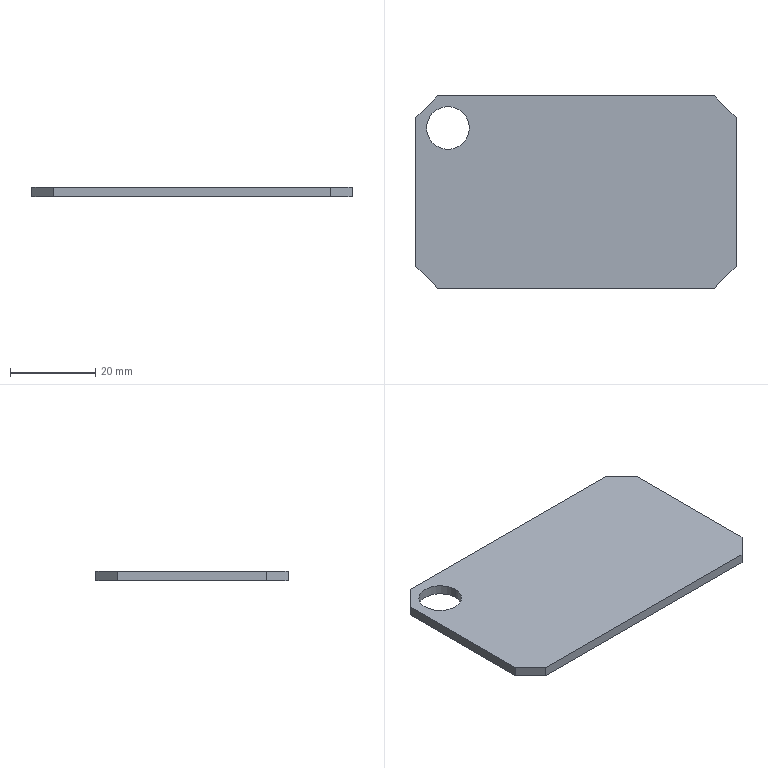Part | STEP file | [20]-1 | 1 solid | 12 faces | box 75 x 45 x 2.3 mm | volume 7467 mm3 | plane 10 | cylinder 2 | commonest cylinder face diameters 10 x2
STEP:
#1=CARTESIAN_POINT('',(2.5,37.5,0.));
#2=VERTEX_POINT('',#1);
#3=CARTESIAN_POINT('',(12.5,37.5,0.));
#4=VERTEX_POINT('',#3);
#5=CARTESIAN_POINT('',(7.5,37.5,0.));
#6=DIRECTION('',(0.,0.,1.));
#7=DIRECTION('',(1.,0.,0.));
#8=AXIS2_PLACEMENT_3D('',#5,#6,#7);
#9=CIRCLE('',#8,5.);
#10=EDGE_CURVE('',#2,#4,#9,.T.);
#11=ORIENTED_EDGE('',*,*,#10,.F.);
#12=CARTESIAN_POINT('',(2.5,37.5,2.3));
#13=VERTEX_POINT('',#12);
#14=CARTESIAN_POINT('',(2.5,37.5,0.));
#15=DIRECTION('',(0.,0.,1.));
#16=VECTOR('',#15,1000.);
#17=LINE('',#14,#16);
#18=EDGE_CURVE('',#2,#13,#17,.T.);
#19=ORIENTED_EDGE('',*,*,#18,.T.);
#20=CARTESIAN_POINT('',(12.5,37.5,2.3));
#21=VERTEX_POINT('',#20);
#22=CARTESIAN_POINT('',(7.5,37.5,2.3));
#23=DIRECTION('',(0.,0.,-1.));
#24=DIRECTION('',(-1.,0.,0.));
#25=AXIS2_PLACEMENT_3D('',#22,#23,#24);
#26=CIRCLE('',#25,5.);
#27=EDGE_CURVE('',#21,#13,#26,.T.);
#28=ORIENTED_EDGE('',*,*,#27,.F.);
#29=CARTESIAN_POINT('',(12.5,37.5,0.));
#30=DIRECTION('',(0.,0.,1.));
#31=VECTOR('',#30,1000.);
#32=LINE('',#29,#31);
#33=EDGE_CURVE('',#4,#21,#32,.T.);
#34=ORIENTED_EDGE('',*,*,#33,.F.);
#35=EDGE_LOOP('',(#11,#19,#28,#34));
#36=FACE_OUTER_BOUND('',#35,.T.);
#37=CARTESIAN_POINT('',(7.5,37.5,0.));
#38=DIRECTION('',(0.,0.,1.));
#39=DIRECTION('',(1.,0.,0.));
#40=AXIS2_PLACEMENT_3D('',#37,#38,#39);
#41=CYLINDRICAL_SURFACE('',#40,5.);
#42=ADVANCED_FACE('',(#36),#41,.F.);
#43=ORIENTED_EDGE('',*,*,#27,.T.);
#44=CARTESIAN_POINT('',(7.5,37.5,2.3));
#45=DIRECTION('',(0.,0.,-1.));
#46=DIRECTION('',(-1.,0.,0.));
#47=AXIS2_PLACEMENT_3D('',#44,#45,#46);
#48=CIRCLE('',#47,5.);
#49=EDGE_CURVE('',#13,#21,#48,.T.);
#50=ORIENTED_EDGE('',*,*,#49,.T.);
#51=EDGE_LOOP('',(#43,#50));
#52=FACE_BOUND('',#51,.T.);
#53=CARTESIAN_POINT('',(0.,5.,2.3));
#54=VERTEX_POINT('',#53);
#55=CARTESIAN_POINT('',(0.,40.,2.3));
#56=VERTEX_POINT('',#55);
#57=CARTESIAN_POINT('',(0.,22.5,2.3));
#58=DIRECTION('',(0.,1.,0.));
#59=VECTOR('',#58,1000.);
#60=LINE('',#57,#59);
#61=EDGE_CURVE('',#54,#56,#60,.T.);
#62=ORIENTED_EDGE('',*,*,#61,.F.);
#63=CARTESIAN_POINT('',(5.,0.,2.3));
#64=VERTEX_POINT('',#63);
#65=CARTESIAN_POINT('',(10.,-5.,2.3));
#66=DIRECTION('',(0.7071,-0.7071,0.));
#67=VECTOR('',#66,1000.);
#68=LINE('',#65,#67);
#69=EDGE_CURVE('',#54,#64,#68,.T.);
#70=ORIENTED_EDGE('',*,*,#69,.T.);
#71=CARTESIAN_POINT('',(70.,0.,2.3));
#72=VERTEX_POINT('',#71);
#73=CARTESIAN_POINT('',(37.5,0.,2.3));
#74=DIRECTION('',(-1.,0.,0.));
#75=VECTOR('',#74,1000.);
#76=LINE('',#73,#75);
#77=EDGE_CURVE('',#72,#64,#76,.T.);
#78=ORIENTED_EDGE('',*,*,#77,.F.);
#79=CARTESIAN_POINT('',(75.,5.,2.3));
#80=VERTEX_POINT('',#79);
#81=CARTESIAN_POINT('',(65.,-5.,2.3));
#82=DIRECTION('',(0.7071,0.7071,0.));
#83=VECTOR('',#82,1000.);
#84=LINE('',#81,#83);
#85=EDGE_CURVE('',#72,#80,#84,.T.);
#86=ORIENTED_EDGE('',*,*,#85,.T.);
#87=CARTESIAN_POINT('',(75.,40.,2.3));
#88=VERTEX_POINT('',#87);
#89=CARTESIAN_POINT('',(75.,22.5,2.3));
#90=DIRECTION('',(0.,-1.,0.));
#91=VECTOR('',#90,1000.);
#92=LINE('',#89,#91);
#93=EDGE_CURVE('',#88,#80,#92,.T.);
#94=ORIENTED_EDGE('',*,*,#93,.F.);
#95=CARTESIAN_POINT('',(70.,45.,2.3));
#96=VERTEX_POINT('',#95);
#97=CARTESIAN_POINT('',(65.,50.,2.3));
#98=DIRECTION('',(-0.7071,0.7071,0.));
#99=VECTOR('',#98,1000.);
#100=LINE('',#97,#99);
#101=EDGE_CURVE('',#88,#96,#100,.T.);
#102=ORIENTED_EDGE('',*,*,#101,.T.);
#103=CARTESIAN_POINT('',(5.,45.,2.3));
#104=VERTEX_POINT('',#103);
#105=CARTESIAN_POINT('',(37.5,45.,2.3));
#106=DIRECTION('',(1.,0.,0.));
#107=VECTOR('',#106,1000.);
#108=LINE('',#105,#107);
#109=EDGE_CURVE('',#104,#96,#108,.T.);
#110=ORIENTED_EDGE('',*,*,#109,.F.);
#111=CARTESIAN_POINT('',(10.,50.,2.3));
#112=DIRECTION('',(-0.7071,-0.7071,0.));
#113=VECTOR('',#112,1000.);
#114=LINE('',#111,#113);
#115=EDGE_CURVE('',#104,#56,#114,.T.);
#116=ORIENTED_EDGE('',*,*,#115,.T.);
#117=EDGE_LOOP('',(#62,#70,#78,#86,#94,#102,#110,#116));
#118=FACE_OUTER_BOUND('',#117,.T.);
#119=CARTESIAN_POINT('',(37.5,22.5,2.3));
#120=DIRECTION('',(0.,0.,1.));
#121=DIRECTION('',(0.,1.,0.));
#122=AXIS2_PLACEMENT_3D('',#119,#120,#121);
#123=PLANE('',#122);
#124=ADVANCED_FACE('',(#52,#118),#123,.T.);
#125=CARTESIAN_POINT('',(75.,5.,0.));
#126=VERTEX_POINT('',#125);
#127=CARTESIAN_POINT('',(75.,40.,0.));
#128=VERTEX_POINT('',#127);
#129=CARTESIAN_POINT('',(75.,22.5,0.));
#130=DIRECTION('',(0.,1.,0.));
#131=VECTOR('',#130,1000.);
#132=LINE('',#129,#131);
#133=EDGE_CURVE('',#126,#128,#132,.T.);
#134=ORIENTED_EDGE('',*,*,#133,.T.);
#135=CARTESIAN_POINT('',(75.,40.,0.));
#136=DIRECTION('',(0.,0.,1.));
#137=VECTOR('',#136,1000.);
#138=LINE('',#135,#137);
#139=EDGE_CURVE('',#128,#88,#138,.T.);
#140=ORIENTED_EDGE('',*,*,#139,.T.);
#141=ORIENTED_EDGE('',*,*,#93,.T.);
#142=CARTESIAN_POINT('',(75.,5.,0.));
#143=DIRECTION('',(0.,0.,-1.));
#144=VECTOR('',#143,1000.);
#145=LINE('',#142,#144);
#146=EDGE_CURVE('',#80,#126,#145,.T.);
#147=ORIENTED_EDGE('',*,*,#146,.T.);
#148=EDGE_LOOP('',(#134,#140,#141,#147));
#149=FACE_OUTER_BOUND('',#148,.T.);
#150=CARTESIAN_POINT('',(75.,22.5,0.));
#151=DIRECTION('',(1.,0.,0.));
#152=DIRECTION('',(0.,0.,-1.));
#153=AXIS2_PLACEMENT_3D('',#150,#151,#152);
#154=PLANE('',#153);
#155=ADVANCED_FACE('',(#149),#154,.T.);
#156=ORIENTED_EDGE('',*,*,#77,.T.);
#157=CARTESIAN_POINT('',(5.,0.,0.));
#158=VERTEX_POINT('',#157);
#159=CARTESIAN_POINT('',(5.,0.,0.));
#160=DIRECTION('',(0.,0.,-1.));
#161=VECTOR('',#160,1000.);
#162=LINE('',#159,#161);
#163=EDGE_CURVE('',#64,#158,#162,.T.);
#164=ORIENTED_EDGE('',*,*,#163,.T.);
#165=CARTESIAN_POINT('',(70.,0.,0.));
#166=VERTEX_POINT('',#165);
#167=CARTESIAN_POINT('',(37.5,0.,0.));
#168=DIRECTION('',(1.,0.,0.));
#169=VECTOR('',#168,1000.);
#170=LINE('',#167,#169);
#171=EDGE_CURVE('',#158,#166,#170,.T.);
#172=ORIENTED_EDGE('',*,*,#171,.T.);
#173=CARTESIAN_POINT('',(70.,0.,0.));
#174=DIRECTION('',(0.,0.,1.));
#175=VECTOR('',#174,1000.);
#176=LINE('',#173,#175);
#177=EDGE_CURVE('',#166,#72,#176,.T.);
#178=ORIENTED_EDGE('',*,*,#177,.T.);
#179=EDGE_LOOP('',(#156,#164,#172,#178));
#180=FACE_OUTER_BOUND('',#179,.T.);
#181=CARTESIAN_POINT('',(37.5,0.,0.));
#182=DIRECTION('',(0.,-1.,0.));
#183=DIRECTION('',(0.,0.,1.));
#184=AXIS2_PLACEMENT_3D('',#181,#182,#183);
#185=PLANE('',#184);
#186=ADVANCED_FACE('',(#180),#185,.T.);
#187=CARTESIAN_POINT('',(0.,40.,0.));
#188=VERTEX_POINT('',#187);
#189=CARTESIAN_POINT('',(0.,5.,0.));
#190=VERTEX_POINT('',#189);
#191=CARTESIAN_POINT('',(0.,22.5,0.));
#192=DIRECTION('',(0.,-1.,0.));
#193=VECTOR('',#192,1000.);
#194=LINE('',#191,#193);
#195=EDGE_CURVE('',#188,#190,#194,.T.);
#196=ORIENTED_EDGE('',*,*,#195,.T.);
#197=CARTESIAN_POINT('',(0.,5.,0.));
#198=DIRECTION('',(0.,0.,1.));
#199=VECTOR('',#198,1000.);
#200=LINE('',#197,#199);
#201=EDGE_CURVE('',#190,#54,#200,.T.);
#202=ORIENTED_EDGE('',*,*,#201,.T.);
#203=ORIENTED_EDGE('',*,*,#61,.T.);
#204=CARTESIAN_POINT('',(0.,40.,0.));
#205=DIRECTION('',(0.,0.,-1.));
#206=VECTOR('',#205,1000.);
#207=LINE('',#204,#206);
#208=EDGE_CURVE('',#56,#188,#207,.T.);
#209=ORIENTED_EDGE('',*,*,#208,.T.);
#210=EDGE_LOOP('',(#196,#202,#203,#209));
#211=FACE_OUTER_BOUND('',#210,.T.);
#212=CARTESIAN_POINT('',(0.,22.5,0.));
#213=DIRECTION('',(-1.,0.,0.));
#214=DIRECTION('',(0.,0.,1.));
#215=AXIS2_PLACEMENT_3D('',#212,#213,#214);
#216=PLANE('',#215);
#217=ADVANCED_FACE('',(#211),#216,.T.);
#218=CARTESIAN_POINT('',(7.5,37.5,0.));
#219=DIRECTION('',(0.,0.,1.));
#220=DIRECTION('',(1.,0.,0.));
#221=AXIS2_PLACEMENT_3D('',#218,#219,#220);
#222=CIRCLE('',#221,5.);
#223=EDGE_CURVE('',#4,#2,#222,.T.);
#224=ORIENTED_EDGE('',*,*,#223,.T.);
#225=ORIENTED_EDGE('',*,*,#10,.T.);
#226=EDGE_LOOP('',(#224,#225));
#227=FACE_BOUND('',#226,.T.);
#228=ORIENTED_EDGE('',*,*,#171,.F.);
#229=CARTESIAN_POINT('',(10.,-5.,0.));
#230=DIRECTION('',(-0.7071,0.7071,0.));
#231=VECTOR('',#230,1000.);
#232=LINE('',#229,#231);
#233=EDGE_CURVE('',#158,#190,#232,.T.);
#234=ORIENTED_EDGE('',*,*,#233,.T.);
#235=ORIENTED_EDGE('',*,*,#195,.F.);
#236=CARTESIAN_POINT('',(5.,45.,0.));
#237=VERTEX_POINT('',#236);
#238=CARTESIAN_POINT('',(10.,50.,0.));
#239=DIRECTION('',(0.7071,0.7071,0.));
#240=VECTOR('',#239,1000.);
#241=LINE('',#238,#240);
#242=EDGE_CURVE('',#188,#237,#241,.T.);
#243=ORIENTED_EDGE('',*,*,#242,.T.);
#244=CARTESIAN_POINT('',(70.,45.,0.));
#245=VERTEX_POINT('',#244);
#246=CARTESIAN_POINT('',(37.5,45.,0.));
#247=DIRECTION('',(-1.,0.,0.));
#248=VECTOR('',#247,1000.);
#249=LINE('',#246,#248);
#250=EDGE_CURVE('',#245,#237,#249,.T.);
#251=ORIENTED_EDGE('',*,*,#250,.F.);
#252=CARTESIAN_POINT('',(65.,50.,0.));
#253=DIRECTION('',(0.7071,-0.7071,0.));
#254=VECTOR('',#253,1000.);
#255=LINE('',#252,#254);
#256=EDGE_CURVE('',#245,#128,#255,.T.);
#257=ORIENTED_EDGE('',*,*,#256,.T.);
#258=ORIENTED_EDGE('',*,*,#133,.F.);
#259=CARTESIAN_POINT('',(65.,-5.,0.));
#260=DIRECTION('',(-0.7071,-0.7071,0.));
#261=VECTOR('',#260,1000.);
#262=LINE('',#259,#261);
#263=EDGE_CURVE('',#126,#166,#262,.T.);
#264=ORIENTED_EDGE('',*,*,#263,.T.);
#265=EDGE_LOOP('',(#228,#234,#235,#243,#251,#257,#258,#264));
#266=FACE_OUTER_BOUND('',#265,.T.);
#267=CARTESIAN_POINT('',(37.5,22.5,0.));
#268=DIRECTION('',(0.,0.,-1.));
#269=DIRECTION('',(0.,-1.,0.));
#270=AXIS2_PLACEMENT_3D('',#267,#268,#269);
#271=PLANE('',#270);
#272=ADVANCED_FACE('',(#227,#266),#271,.T.);
#273=ORIENTED_EDGE('',*,*,#250,.T.);
#274=CARTESIAN_POINT('',(5.,45.,0.));
#275=DIRECTION('',(0.,0.,1.));
#276=VECTOR('',#275,1000.);
#277=LINE('',#274,#276);
#278=EDGE_CURVE('',#237,#104,#277,.T.);
#279=ORIENTED_EDGE('',*,*,#278,.T.);
#280=ORIENTED_EDGE('',*,*,#109,.T.);
#281=CARTESIAN_POINT('',(70.,45.,0.));
#282=DIRECTION('',(0.,0.,-1.));
#283=VECTOR('',#282,1000.);
#284=LINE('',#281,#283);
#285=EDGE_CURVE('',#96,#245,#284,.T.);
#286=ORIENTED_EDGE('',*,*,#285,.T.);
#287=EDGE_LOOP('',(#273,#279,#280,#286));
#288=FACE_OUTER_BOUND('',#287,.T.);
#289=CARTESIAN_POINT('',(37.5,45.,0.));
#290=DIRECTION('',(0.,1.,0.));
#291=DIRECTION('',(0.,0.,-1.));
#292=AXIS2_PLACEMENT_3D('',#289,#290,#291);
#293=PLANE('',#292);
#294=ADVANCED_FACE('',(#288),#293,.T.);
#295=ORIENTED_EDGE('',*,*,#256,.F.);
#296=ORIENTED_EDGE('',*,*,#285,.F.);
#297=ORIENTED_EDGE('',*,*,#101,.F.);
#298=ORIENTED_EDGE('',*,*,#139,.F.);
#299=EDGE_LOOP('',(#295,#296,#297,#298));
#300=FACE_OUTER_BOUND('',#299,.T.);
#301=CARTESIAN_POINT('',(75.,40.,0.));
#302=DIRECTION('',(-0.7071,-0.7071,0.));
#303=DIRECTION('',(0.,0.,1.));
#304=AXIS2_PLACEMENT_3D('',#301,#302,#303);
#305=PLANE('',#304);
#306=ADVANCED_FACE('',(#300),#305,.F.);
#307=ORIENTED_EDGE('',*,*,#263,.F.);
#308=ORIENTED_EDGE('',*,*,#146,.F.);
#309=ORIENTED_EDGE('',*,*,#85,.F.);
#310=ORIENTED_EDGE('',*,*,#177,.F.);
#311=EDGE_LOOP('',(#307,#308,#309,#310));
#312=FACE_OUTER_BOUND('',#311,.T.);
#313=CARTESIAN_POINT('',(70.,0.,0.));
#314=DIRECTION('',(-0.7071,0.7071,0.));
#315=DIRECTION('',(0.,0.,1.));
#316=AXIS2_PLACEMENT_3D('',#313,#314,#315);
#317=PLANE('',#316);
#318=ADVANCED_FACE('',(#312),#317,.F.);
#319=ORIENTED_EDGE('',*,*,#233,.F.);
#320=ORIENTED_EDGE('',*,*,#163,.F.);
#321=ORIENTED_EDGE('',*,*,#69,.F.);
#322=ORIENTED_EDGE('',*,*,#201,.F.);
#323=EDGE_LOOP('',(#319,#320,#321,#322));
#324=FACE_OUTER_BOUND('',#323,.T.);
#325=CARTESIAN_POINT('',(0.,5.,0.));
#326=DIRECTION('',(0.7071,0.7071,0.));
#327=DIRECTION('',(0.,0.,1.));
#328=AXIS2_PLACEMENT_3D('',#325,#326,#327);
#329=PLANE('',#328);
#330=ADVANCED_FACE('',(#324),#329,.F.);
#331=ORIENTED_EDGE('',*,*,#242,.F.);
#332=ORIENTED_EDGE('',*,*,#208,.F.);
#333=ORIENTED_EDGE('',*,*,#115,.F.);
#334=ORIENTED_EDGE('',*,*,#278,.F.);
#335=EDGE_LOOP('',(#331,#332,#333,#334));
#336=FACE_OUTER_BOUND('',#335,.T.);
#337=CARTESIAN_POINT('',(5.,45.,0.));
#338=DIRECTION('',(0.7071,-0.7071,0.));
#339=DIRECTION('',(0.,0.,1.));
#340=AXIS2_PLACEMENT_3D('',#337,#338,#339);
#341=PLANE('',#340);
#342=ADVANCED_FACE('',(#336),#341,.F.);
#343=ORIENTED_EDGE('',*,*,#18,.F.);
#344=ORIENTED_EDGE('',*,*,#223,.F.);
#345=ORIENTED_EDGE('',*,*,#33,.T.);
#346=ORIENTED_EDGE('',*,*,#49,.F.);
#347=EDGE_LOOP('',(#343,#344,#345,#346));
#348=FACE_OUTER_BOUND('',#347,.T.);
#349=CARTESIAN_POINT('',(7.5,37.5,0.));
#350=DIRECTION('',(0.,0.,1.));
#351=DIRECTION('',(1.,0.,0.));
#352=AXIS2_PLACEMENT_3D('',#349,#350,#351);
#353=CYLINDRICAL_SURFACE('',#352,5.);
#354=ADVANCED_FACE('',(#348),#353,.F.);
#355=CLOSED_SHELL('',(#42,#124,#155,#186,#217,#272,#294,#306,#318,#330,#342,#354));
#356=MANIFOLD_SOLID_BREP('',#355);
#357=CARTESIAN_POINT('',(0.,0.,0.));
#358=DIRECTION('',(0.,0.,1.));
#359=DIRECTION('',(1.,0.,0.));
#360=AXIS2_PLACEMENT_3D('',#357,#358,#359);
#361=(LENGTH_UNIT()NAMED_UNIT(*)SI_UNIT(.MILLI.,.METRE.));
#362=UNCERTAINTY_MEASURE_WITH_UNIT(LENGTH_MEASURE(0.00001),#361,'','');
#363=(NAMED_UNIT(*)PLANE_ANGLE_UNIT()SI_UNIT($,.RADIAN.));
#364=(NAMED_UNIT(*)SI_UNIT($,.STERADIAN.)SOLID_ANGLE_UNIT());
#365=(GEOMETRIC_REPRESENTATION_CONTEXT(3)GLOBAL_UNCERTAINTY_ASSIGNED_CONTEXT((#362))GLOBAL_UNIT_ASSIGNED_CONTEXT((#361,#363,#364))REPRESENTATION_CONTEXT('',''));
#366=ADVANCED_BREP_SHAPE_REPRESENTATION('',(#356,#360),#365);